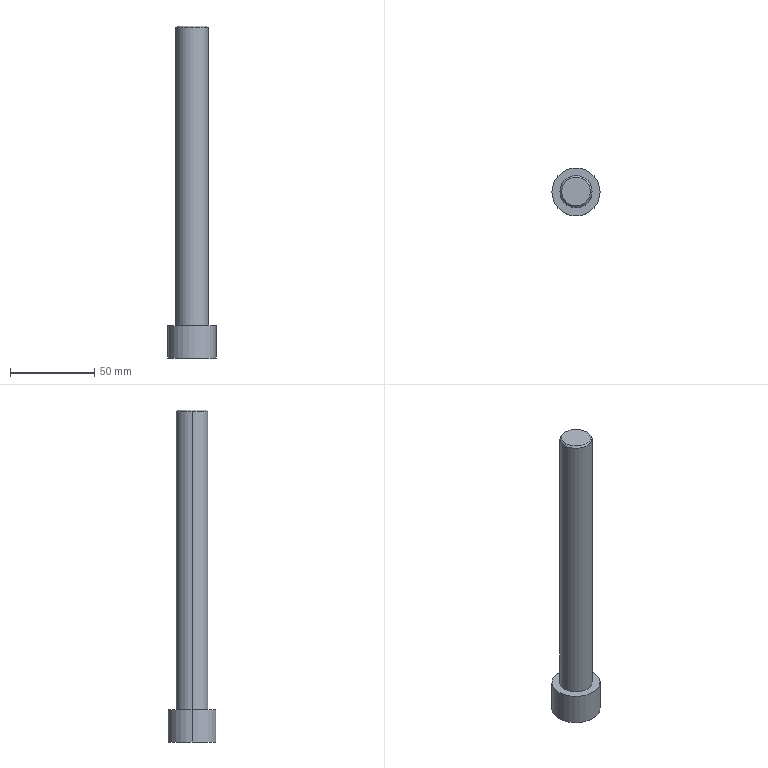Part | STEP file | 4-20.sldasm-Part-315 | 1 solid | 16 faces | box 28.575 x 28.575 x 196.85 mm | volume 60119 mm3 | plane 10 | cylinder 4 | cone 2 | commonest cylinder face diameters 19.05 x2 28.575 x2
STEP:
#1=CARTESIAN_POINT('',(193.494,418.,17.099));
#2=VERTEX_POINT('',#1);
#3=CARTESIAN_POINT('',(176.506,418.,17.099));
#4=VERTEX_POINT('',#3);
#5=CARTESIAN_POINT('',(185.,418.,17.099));
#6=DIRECTION('',(0.,0.,-1.));
#7=DIRECTION('',(1.,0.,0.));
#8=AXIS2_PLACEMENT_3D('',#5,#6,#7);
#9=CIRCLE('',#8,8.494);
#10=EDGE_CURVE('',#2,#4,#9,.T.);
#11=ORIENTED_EDGE('',*,*,#10,.T.);
#12=CARTESIAN_POINT('',(175.475,418.,16.068));
#13=VERTEX_POINT('',#12);
#14=CARTESIAN_POINT('',(175.475,418.,16.068));
#15=DIRECTION('',(-0.7071,0.,-0.7071));
#16=VECTOR('',#15,1000.);
#17=LINE('',#14,#16);
#18=EDGE_CURVE('',#4,#13,#17,.T.);
#19=ORIENTED_EDGE('',*,*,#18,.T.);
#20=CARTESIAN_POINT('',(194.525,418.,16.068));
#21=VERTEX_POINT('',#20);
#22=CARTESIAN_POINT('',(185.,418.,16.068));
#23=DIRECTION('',(0.,0.,1.));
#24=DIRECTION('',(1.,0.,0.));
#25=AXIS2_PLACEMENT_3D('',#22,#23,#24);
#26=CIRCLE('',#25,9.525);
#27=EDGE_CURVE('',#13,#21,#26,.T.);
#28=ORIENTED_EDGE('',*,*,#27,.T.);
#29=CARTESIAN_POINT('',(194.525,418.,16.068));
#30=DIRECTION('',(0.7071,0.,-0.7071));
#31=VECTOR('',#30,1000.);
#32=LINE('',#29,#31);
#33=EDGE_CURVE('',#2,#21,#32,.T.);
#34=ORIENTED_EDGE('',*,*,#33,.F.);
#35=EDGE_LOOP('',(#11,#19,#28,#34));
#36=FACE_OUTER_BOUND('',#35,.T.);
#37=CARTESIAN_POINT('',(185.,418.,16.068));
#38=DIRECTION('',(0.,0.,-1.));
#39=DIRECTION('',(1.,0.,0.));
#40=AXIS2_PLACEMENT_3D('',#37,#38,#39);
#41=CONICAL_SURFACE('',#40,9.525,0.7854);
#42=ADVANCED_FACE('',(#36),#41,.T.);
#43=CARTESIAN_POINT('',(170.712,418.,-160.701));
#44=VERTEX_POINT('',#43);
#45=CARTESIAN_POINT('',(199.287,418.,-160.701));
#46=VERTEX_POINT('',#45);
#47=CARTESIAN_POINT('',(185.,418.,-160.701));
#48=DIRECTION('',(0.,0.,1.));
#49=DIRECTION('',(1.,0.,0.));
#50=AXIS2_PLACEMENT_3D('',#47,#48,#49);
#51=CIRCLE('',#50,14.288);
#52=EDGE_CURVE('',#44,#46,#51,.T.);
#53=ORIENTED_EDGE('',*,*,#52,.F.);
#54=CARTESIAN_POINT('',(170.712,418.,-179.751));
#55=VERTEX_POINT('',#54);
#56=CARTESIAN_POINT('',(170.712,418.,-160.701));
#57=DIRECTION('',(0.,0.,-1.));
#58=VECTOR('',#57,1000.);
#59=LINE('',#56,#58);
#60=EDGE_CURVE('',#44,#55,#59,.T.);
#61=ORIENTED_EDGE('',*,*,#60,.T.);
#62=CARTESIAN_POINT('',(199.287,418.,-179.751));
#63=VERTEX_POINT('',#62);
#64=CARTESIAN_POINT('',(185.,418.,-179.751));
#65=DIRECTION('',(0.,0.,1.));
#66=DIRECTION('',(1.,0.,0.));
#67=AXIS2_PLACEMENT_3D('',#64,#65,#66);
#68=CIRCLE('',#67,14.288);
#69=EDGE_CURVE('',#55,#63,#68,.T.);
#70=ORIENTED_EDGE('',*,*,#69,.T.);
#71=CARTESIAN_POINT('',(199.287,418.,-160.701));
#72=DIRECTION('',(0.,0.,-1.));
#73=VECTOR('',#72,1000.);
#74=LINE('',#71,#73);
#75=EDGE_CURVE('',#46,#63,#74,.T.);
#76=ORIENTED_EDGE('',*,*,#75,.F.);
#77=EDGE_LOOP('',(#53,#61,#70,#76));
#78=FACE_OUTER_BOUND('',#77,.T.);
#79=CARTESIAN_POINT('',(185.,418.,-160.701));
#80=DIRECTION('',(0.,0.,-1.));
#81=DIRECTION('',(1.,0.,0.));
#82=AXIS2_PLACEMENT_3D('',#79,#80,#81);
#83=CYLINDRICAL_SURFACE('',#82,14.288);
#84=ADVANCED_FACE('',(#78),#83,.T.);
#85=CARTESIAN_POINT('',(175.475,418.,-160.701));
#86=VERTEX_POINT('',#85);
#87=CARTESIAN_POINT('',(194.525,418.,-160.701));
#88=VERTEX_POINT('',#87);
#89=CARTESIAN_POINT('',(185.,418.,-160.701));
#90=DIRECTION('',(0.,0.,1.));
#91=DIRECTION('',(1.,0.,0.));
#92=AXIS2_PLACEMENT_3D('',#89,#90,#91);
#93=CIRCLE('',#92,9.525);
#94=EDGE_CURVE('',#86,#88,#93,.T.);
#95=ORIENTED_EDGE('',*,*,#94,.T.);
#96=CARTESIAN_POINT('',(194.525,418.,-160.701));
#97=DIRECTION('',(0.,0.,1.));
#98=VECTOR('',#97,1000.);
#99=LINE('',#96,#98);
#100=EDGE_CURVE('',#88,#21,#99,.T.);
#101=ORIENTED_EDGE('',*,*,#100,.T.);
#102=ORIENTED_EDGE('',*,*,#27,.F.);
#103=CARTESIAN_POINT('',(175.475,418.,-160.701));
#104=DIRECTION('',(0.,0.,1.));
#105=VECTOR('',#104,1000.);
#106=LINE('',#103,#105);
#107=EDGE_CURVE('',#86,#13,#106,.T.);
#108=ORIENTED_EDGE('',*,*,#107,.F.);
#109=EDGE_LOOP('',(#95,#101,#102,#108));
#110=FACE_OUTER_BOUND('',#109,.T.);
#111=CARTESIAN_POINT('',(185.,418.,-160.701));
#112=DIRECTION('',(0.,0.,1.));
#113=DIRECTION('',(-1.,0.,0.));
#114=AXIS2_PLACEMENT_3D('',#111,#112,#113);
#115=CYLINDRICAL_SURFACE('',#114,9.525);
#116=ADVANCED_FACE('',(#110),#115,.T.);
#117=ORIENTED_EDGE('',*,*,#100,.F.);
#118=CARTESIAN_POINT('',(185.,418.,-160.701));
#119=DIRECTION('',(0.,0.,1.));
#120=DIRECTION('',(1.,0.,0.));
#121=AXIS2_PLACEMENT_3D('',#118,#119,#120);
#122=CIRCLE('',#121,9.525);
#123=EDGE_CURVE('',#88,#86,#122,.T.);
#124=ORIENTED_EDGE('',*,*,#123,.T.);
#125=ORIENTED_EDGE('',*,*,#107,.T.);
#126=CARTESIAN_POINT('',(185.,418.,16.068));
#127=DIRECTION('',(0.,0.,1.));
#128=DIRECTION('',(1.,0.,0.));
#129=AXIS2_PLACEMENT_3D('',#126,#127,#128);
#130=CIRCLE('',#129,9.525);
#131=EDGE_CURVE('',#21,#13,#130,.T.);
#132=ORIENTED_EDGE('',*,*,#131,.F.);
#133=EDGE_LOOP('',(#117,#124,#125,#132));
#134=FACE_OUTER_BOUND('',#133,.T.);
#135=CARTESIAN_POINT('',(185.,418.,-160.701));
#136=DIRECTION('',(0.,0.,1.));
#137=DIRECTION('',(-1.,0.,0.));
#138=AXIS2_PLACEMENT_3D('',#135,#136,#137);
#139=CYLINDRICAL_SURFACE('',#138,9.525);
#140=ADVANCED_FACE('',(#134),#139,.T.);
#141=ORIENTED_EDGE('',*,*,#10,.F.);
#142=CARTESIAN_POINT('',(185.,418.,17.099));
#143=DIRECTION('',(0.,0.,-1.));
#144=DIRECTION('',(1.,0.,0.));
#145=AXIS2_PLACEMENT_3D('',#142,#143,#144);
#146=CIRCLE('',#145,8.494);
#147=EDGE_CURVE('',#4,#2,#146,.T.);
#148=ORIENTED_EDGE('',*,*,#147,.F.);
#149=EDGE_LOOP('',(#141,#148));
#150=FACE_OUTER_BOUND('',#149,.T.);
#151=CARTESIAN_POINT('',(185.,418.,17.099));
#152=DIRECTION('',(0.,0.,-1.));
#153=DIRECTION('',(1.,0.,0.));
#154=AXIS2_PLACEMENT_3D('',#151,#152,#153);
#155=PLANE('',#154);
#156=ADVANCED_FACE('',(#150),#155,.F.);
#157=CARTESIAN_POINT('',(185.,418.,-160.701));
#158=DIRECTION('',(0.,0.,1.));
#159=DIRECTION('',(1.,0.,0.));
#160=AXIS2_PLACEMENT_3D('',#157,#158,#159);
#161=CIRCLE('',#160,14.288);
#162=EDGE_CURVE('',#46,#44,#161,.T.);
#163=ORIENTED_EDGE('',*,*,#162,.T.);
#164=ORIENTED_EDGE('',*,*,#52,.T.);
#165=EDGE_LOOP('',(#163,#164));
#166=FACE_OUTER_BOUND('',#165,.T.);
#167=ORIENTED_EDGE('',*,*,#94,.F.);
#168=ORIENTED_EDGE('',*,*,#123,.F.);
#169=EDGE_LOOP('',(#167,#168));
#170=FACE_BOUND('',#169,.T.);
#171=CARTESIAN_POINT('',(185.,418.,-160.701));
#172=DIRECTION('',(0.,0.,1.));
#173=DIRECTION('',(-1.,0.,0.));
#174=AXIS2_PLACEMENT_3D('',#171,#172,#173);
#175=PLANE('',#174);
#176=ADVANCED_FACE('',(#166,#170),#175,.T.);
#177=CARTESIAN_POINT('',(180.417,410.062,-179.751));
#178=VERTEX_POINT('',#177);
#179=CARTESIAN_POINT('',(189.583,410.062,-179.751));
#180=VERTEX_POINT('',#179);
#181=CARTESIAN_POINT('',(180.417,410.062,-179.751));
#182=DIRECTION('',(1.,0.,0.));
#183=VECTOR('',#182,1000.);
#184=LINE('',#181,#183);
#185=EDGE_CURVE('',#178,#180,#184,.T.);
#186=ORIENTED_EDGE('',*,*,#185,.T.);
#187=CARTESIAN_POINT('',(194.165,418.,-179.751));
#188=VERTEX_POINT('',#187);
#189=CARTESIAN_POINT('',(189.583,410.062,-179.751));
#190=DIRECTION('',(0.5,0.866,0.));
#191=VECTOR('',#190,1000.);
#192=LINE('',#189,#191);
#193=EDGE_CURVE('',#180,#188,#192,.T.);
#194=ORIENTED_EDGE('',*,*,#193,.T.);
#195=CARTESIAN_POINT('',(189.583,425.938,-179.751));
#196=VERTEX_POINT('',#195);
#197=CARTESIAN_POINT('',(194.165,418.,-179.751));
#198=DIRECTION('',(-0.5,0.866,0.));
#199=VECTOR('',#198,1000.);
#200=LINE('',#197,#199);
#201=EDGE_CURVE('',#188,#196,#200,.T.);
#202=ORIENTED_EDGE('',*,*,#201,.T.);
#203=CARTESIAN_POINT('',(180.417,425.938,-179.751));
#204=VERTEX_POINT('',#203);
#205=CARTESIAN_POINT('',(189.583,425.938,-179.751));
#206=DIRECTION('',(-1.,0.,0.));
#207=VECTOR('',#206,1000.);
#208=LINE('',#205,#207);
#209=EDGE_CURVE('',#196,#204,#208,.T.);
#210=ORIENTED_EDGE('',*,*,#209,.T.);
#211=CARTESIAN_POINT('',(175.835,418.,-179.751));
#212=VERTEX_POINT('',#211);
#213=CARTESIAN_POINT('',(180.417,425.938,-179.751));
#214=DIRECTION('',(-0.5,-0.866,0.));
#215=VECTOR('',#214,1000.);
#216=LINE('',#213,#215);
#217=EDGE_CURVE('',#204,#212,#216,.T.);
#218=ORIENTED_EDGE('',*,*,#217,.T.);
#219=CARTESIAN_POINT('',(175.835,418.,-179.751));
#220=DIRECTION('',(0.5,-0.866,0.));
#221=VECTOR('',#220,1000.);
#222=LINE('',#219,#221);
#223=EDGE_CURVE('',#212,#178,#222,.T.);
#224=ORIENTED_EDGE('',*,*,#223,.T.);
#225=EDGE_LOOP('',(#186,#194,#202,#210,#218,#224));
#226=FACE_BOUND('',#225,.T.);
#227=CARTESIAN_POINT('',(185.,418.,-179.751));
#228=DIRECTION('',(0.,0.,1.));
#229=DIRECTION('',(1.,0.,0.));
#230=AXIS2_PLACEMENT_3D('',#227,#228,#229);
#231=CIRCLE('',#230,14.288);
#232=EDGE_CURVE('',#63,#55,#231,.T.);
#233=ORIENTED_EDGE('',*,*,#232,.F.);
#234=ORIENTED_EDGE('',*,*,#69,.F.);
#235=EDGE_LOOP('',(#233,#234));
#236=FACE_OUTER_BOUND('',#235,.T.);
#237=CARTESIAN_POINT('',(185.,418.,-179.751));
#238=DIRECTION('',(0.,0.,-1.));
#239=DIRECTION('',(1.,0.,0.));
#240=AXIS2_PLACEMENT_3D('',#237,#238,#239);
#241=PLANE('',#240);
#242=ADVANCED_FACE('',(#226,#236),#241,.T.);
#243=ORIENTED_EDGE('',*,*,#60,.F.);
#244=ORIENTED_EDGE('',*,*,#162,.F.);
#245=ORIENTED_EDGE('',*,*,#75,.T.);
#246=ORIENTED_EDGE('',*,*,#232,.T.);
#247=EDGE_LOOP('',(#243,#244,#245,#246));
#248=FACE_OUTER_BOUND('',#247,.T.);
#249=CARTESIAN_POINT('',(185.,418.,-160.701));
#250=DIRECTION('',(0.,0.,-1.));
#251=DIRECTION('',(1.,0.,0.));
#252=AXIS2_PLACEMENT_3D('',#249,#250,#251);
#253=CYLINDRICAL_SURFACE('',#252,14.288);
#254=ADVANCED_FACE('',(#248),#253,.T.);
#255=ORIENTED_EDGE('',*,*,#18,.F.);
#256=ORIENTED_EDGE('',*,*,#147,.T.);
#257=ORIENTED_EDGE('',*,*,#33,.T.);
#258=ORIENTED_EDGE('',*,*,#131,.T.);
#259=EDGE_LOOP('',(#255,#256,#257,#258));
#260=FACE_OUTER_BOUND('',#259,.T.);
#261=CARTESIAN_POINT('',(185.,418.,16.068));
#262=DIRECTION('',(0.,0.,-1.));
#263=DIRECTION('',(1.,0.,0.));
#264=AXIS2_PLACEMENT_3D('',#261,#262,#263);
#265=CONICAL_SURFACE('',#264,9.525,0.7854);
#266=ADVANCED_FACE('',(#260),#265,.T.);
#267=ORIENTED_EDGE('',*,*,#185,.F.);
#268=CARTESIAN_POINT('',(180.417,410.062,-167.178));
#269=VERTEX_POINT('',#268);
#270=CARTESIAN_POINT('',(180.417,410.062,-167.178));
#271=DIRECTION('',(0.,0.,-1.));
#272=VECTOR('',#271,1000.);
#273=LINE('',#270,#272);
#274=EDGE_CURVE('',#269,#178,#273,.T.);
#275=ORIENTED_EDGE('',*,*,#274,.F.);
#276=CARTESIAN_POINT('',(189.583,410.062,-167.178));
#277=VERTEX_POINT('',#276);
#278=CARTESIAN_POINT('',(180.417,410.062,-167.178));
#279=DIRECTION('',(1.,0.,0.));
#280=VECTOR('',#279,1000.);
#281=LINE('',#278,#280);
#282=EDGE_CURVE('',#269,#277,#281,.T.);
#283=ORIENTED_EDGE('',*,*,#282,.T.);
#284=CARTESIAN_POINT('',(189.583,410.062,-167.178));
#285=DIRECTION('',(0.,0.,-1.));
#286=VECTOR('',#285,1000.);
#287=LINE('',#284,#286);
#288=EDGE_CURVE('',#277,#180,#287,.T.);
#289=ORIENTED_EDGE('',*,*,#288,.T.);
#290=EDGE_LOOP('',(#267,#275,#283,#289));
#291=FACE_OUTER_BOUND('',#290,.T.);
#292=CARTESIAN_POINT('',(180.417,410.062,-167.178));
#293=DIRECTION('',(0.,-1.,0.));
#294=DIRECTION('',(0.,0.,1.));
#295=AXIS2_PLACEMENT_3D('',#292,#293,#294);
#296=PLANE('',#295);
#297=ADVANCED_FACE('',(#291),#296,.F.);
#298=ORIENTED_EDGE('',*,*,#193,.F.);
#299=ORIENTED_EDGE('',*,*,#288,.F.);
#300=CARTESIAN_POINT('',(194.165,418.,-167.178));
#301=VERTEX_POINT('',#300);
#302=CARTESIAN_POINT('',(189.583,410.062,-167.178));
#303=DIRECTION('',(0.5,0.866,0.));
#304=VECTOR('',#303,1000.);
#305=LINE('',#302,#304);
#306=EDGE_CURVE('',#277,#301,#305,.T.);
#307=ORIENTED_EDGE('',*,*,#306,.T.);
#308=CARTESIAN_POINT('',(194.165,418.,-167.178));
#309=DIRECTION('',(0.,0.,-1.));
#310=VECTOR('',#309,1000.);
#311=LINE('',#308,#310);
#312=EDGE_CURVE('',#301,#188,#311,.T.);
#313=ORIENTED_EDGE('',*,*,#312,.T.);
#314=EDGE_LOOP('',(#298,#299,#307,#313));
#315=FACE_OUTER_BOUND('',#314,.T.);
#316=CARTESIAN_POINT('',(189.583,410.062,-167.178));
#317=DIRECTION('',(0.866,-0.5,0.));
#318=DIRECTION('',(0.5,0.866,0.));
#319=AXIS2_PLACEMENT_3D('',#316,#317,#318);
#320=PLANE('',#319);
#321=ADVANCED_FACE('',(#315),#320,.F.);
#322=ORIENTED_EDGE('',*,*,#201,.F.);
#323=ORIENTED_EDGE('',*,*,#312,.F.);
#324=CARTESIAN_POINT('',(189.583,425.938,-167.178));
#325=VERTEX_POINT('',#324);
#326=CARTESIAN_POINT('',(194.165,418.,-167.178));
#327=DIRECTION('',(-0.5,0.866,0.));
#328=VECTOR('',#327,1000.);
#329=LINE('',#326,#328);
#330=EDGE_CURVE('',#301,#325,#329,.T.);
#331=ORIENTED_EDGE('',*,*,#330,.T.);
#332=CARTESIAN_POINT('',(189.583,425.938,-167.178));
#333=DIRECTION('',(0.,0.,-1.));
#334=VECTOR('',#333,1000.);
#335=LINE('',#332,#334);
#336=EDGE_CURVE('',#325,#196,#335,.T.);
#337=ORIENTED_EDGE('',*,*,#336,.T.);
#338=EDGE_LOOP('',(#322,#323,#331,#337));
#339=FACE_OUTER_BOUND('',#338,.T.);
#340=CARTESIAN_POINT('',(194.165,418.,-167.178));
#341=DIRECTION('',(0.866,0.5,0.));
#342=DIRECTION('',(-0.5,0.866,0.));
#343=AXIS2_PLACEMENT_3D('',#340,#341,#342);
#344=PLANE('',#343);
#345=ADVANCED_FACE('',(#339),#344,.F.);
#346=ORIENTED_EDGE('',*,*,#209,.F.);
#347=ORIENTED_EDGE('',*,*,#336,.F.);
#348=CARTESIAN_POINT('',(180.417,425.938,-167.178));
#349=VERTEX_POINT('',#348);
#350=CARTESIAN_POINT('',(189.583,425.938,-167.178));
#351=DIRECTION('',(-1.,0.,0.));
#352=VECTOR('',#351,1000.);
#353=LINE('',#350,#352);
#354=EDGE_CURVE('',#325,#349,#353,.T.);
#355=ORIENTED_EDGE('',*,*,#354,.T.);
#356=CARTESIAN_POINT('',(180.417,425.938,-167.178));
#357=DIRECTION('',(0.,0.,-1.));
#358=VECTOR('',#357,1000.);
#359=LINE('',#356,#358);
#360=EDGE_CURVE('',#349,#204,#359,.T.);
#361=ORIENTED_EDGE('',*,*,#360,.T.);
#362=EDGE_LOOP('',(#346,#347,#355,#361));
#363=FACE_OUTER_BOUND('',#362,.T.);
#364=CARTESIAN_POINT('',(189.583,425.938,-167.178));
#365=DIRECTION('',(0.,1.,0.));
#366=DIRECTION('',(0.,0.,-1.));
#367=AXIS2_PLACEMENT_3D('',#364,#365,#366);
#368=PLANE('',#367);
#369=ADVANCED_FACE('',(#363),#368,.F.);
#370=ORIENTED_EDGE('',*,*,#217,.F.);
#371=ORIENTED_EDGE('',*,*,#360,.F.);
#372=CARTESIAN_POINT('',(175.835,418.,-167.178));
#373=VERTEX_POINT('',#372);
#374=CARTESIAN_POINT('',(180.417,425.938,-167.178));
#375=DIRECTION('',(-0.5,-0.866,0.));
#376=VECTOR('',#375,1000.);
#377=LINE('',#374,#376);
#378=EDGE_CURVE('',#349,#373,#377,.T.);
#379=ORIENTED_EDGE('',*,*,#378,.T.);
#380=CARTESIAN_POINT('',(175.835,418.,-167.178));
#381=DIRECTION('',(0.,0.,-1.));
#382=VECTOR('',#381,1000.);
#383=LINE('',#380,#382);
#384=EDGE_CURVE('',#373,#212,#383,.T.);
#385=ORIENTED_EDGE('',*,*,#384,.T.);
#386=EDGE_LOOP('',(#370,#371,#379,#385));
#387=FACE_OUTER_BOUND('',#386,.T.);
#388=CARTESIAN_POINT('',(180.417,425.938,-167.178));
#389=DIRECTION('',(-0.866,0.5,0.));
#390=DIRECTION('',(-0.5,-0.866,0.));
#391=AXIS2_PLACEMENT_3D('',#388,#389,#390);
#392=PLANE('',#391);
#393=ADVANCED_FACE('',(#387),#392,.F.);
#394=ORIENTED_EDGE('',*,*,#223,.F.);
#395=ORIENTED_EDGE('',*,*,#384,.F.);
#396=CARTESIAN_POINT('',(175.835,418.,-167.178));
#397=DIRECTION('',(0.5,-0.866,0.));
#398=VECTOR('',#397,1000.);
#399=LINE('',#396,#398);
#400=EDGE_CURVE('',#373,#269,#399,.T.);
#401=ORIENTED_EDGE('',*,*,#400,.T.);
#402=ORIENTED_EDGE('',*,*,#274,.T.);
#403=EDGE_LOOP('',(#394,#395,#401,#402));
#404=FACE_OUTER_BOUND('',#403,.T.);
#405=CARTESIAN_POINT('',(175.835,418.,-167.178));
#406=DIRECTION('',(-0.866,-0.5,0.));
#407=DIRECTION('',(0.5,-0.866,0.));
#408=AXIS2_PLACEMENT_3D('',#405,#406,#407);
#409=PLANE('',#408);
#410=ADVANCED_FACE('',(#404),#409,.F.);
#411=ORIENTED_EDGE('',*,*,#282,.F.);
#412=ORIENTED_EDGE('',*,*,#400,.F.);
#413=ORIENTED_EDGE('',*,*,#378,.F.);
#414=ORIENTED_EDGE('',*,*,#354,.F.);
#415=ORIENTED_EDGE('',*,*,#330,.F.);
#416=ORIENTED_EDGE('',*,*,#306,.F.);
#417=EDGE_LOOP('',(#411,#412,#413,#414,#415,#416));
#418=FACE_OUTER_BOUND('',#417,.T.);
#419=CARTESIAN_POINT('',(189.583,410.062,-167.178));
#420=DIRECTION('',(0.,0.,-1.));
#421=DIRECTION('',(1.,0.,0.));
#422=AXIS2_PLACEMENT_3D('',#419,#420,#421);
#423=PLANE('',#422);
#424=ADVANCED_FACE('',(#418),#423,.T.);
#425=CLOSED_SHELL('',(#42,#84,#116,#140,#156,#176,#242,#254,#266,#297,#321,#345,#369,#393,#410,#424));
#426=MANIFOLD_SOLID_BREP('',#425);
#427=CARTESIAN_POINT('',(0.,0.,0.));
#428=DIRECTION('',(0.,0.,1.));
#429=DIRECTION('',(1.,0.,0.));
#430=AXIS2_PLACEMENT_3D('',#427,#428,#429);
#431=(LENGTH_UNIT()NAMED_UNIT(*)SI_UNIT(.MILLI.,.METRE.));
#432=UNCERTAINTY_MEASURE_WITH_UNIT(LENGTH_MEASURE(0.00001),#431,'','');
#433=(NAMED_UNIT(*)PLANE_ANGLE_UNIT()SI_UNIT($,.RADIAN.));
#434=(NAMED_UNIT(*)SI_UNIT($,.STERADIAN.)SOLID_ANGLE_UNIT());
#435=(GEOMETRIC_REPRESENTATION_CONTEXT(3)GLOBAL_UNCERTAINTY_ASSIGNED_CONTEXT((#432))GLOBAL_UNIT_ASSIGNED_CONTEXT((#431,#433,#434))REPRESENTATION_CONTEXT('',''));
#436=ADVANCED_BREP_SHAPE_REPRESENTATION('',(#426,#430),#435);